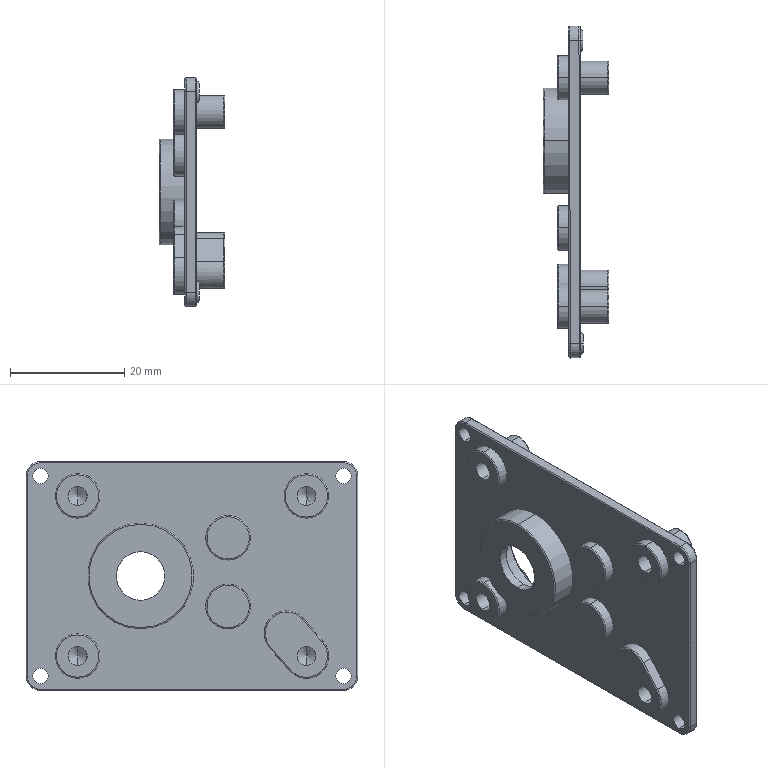Part | SolidWorks | features BaseBody 1 | 1 solid | 145 faces | box 11.539 x 58.002 x 40 mm | volume 5737 mm3 | cylinder 66 | torus 40 | plane 29 | cone 10 | commonest cylinder face diameters 7.8 x13 0.4 x12 5.8 x9 2.7 x8 3.3 x8 2.5 x6